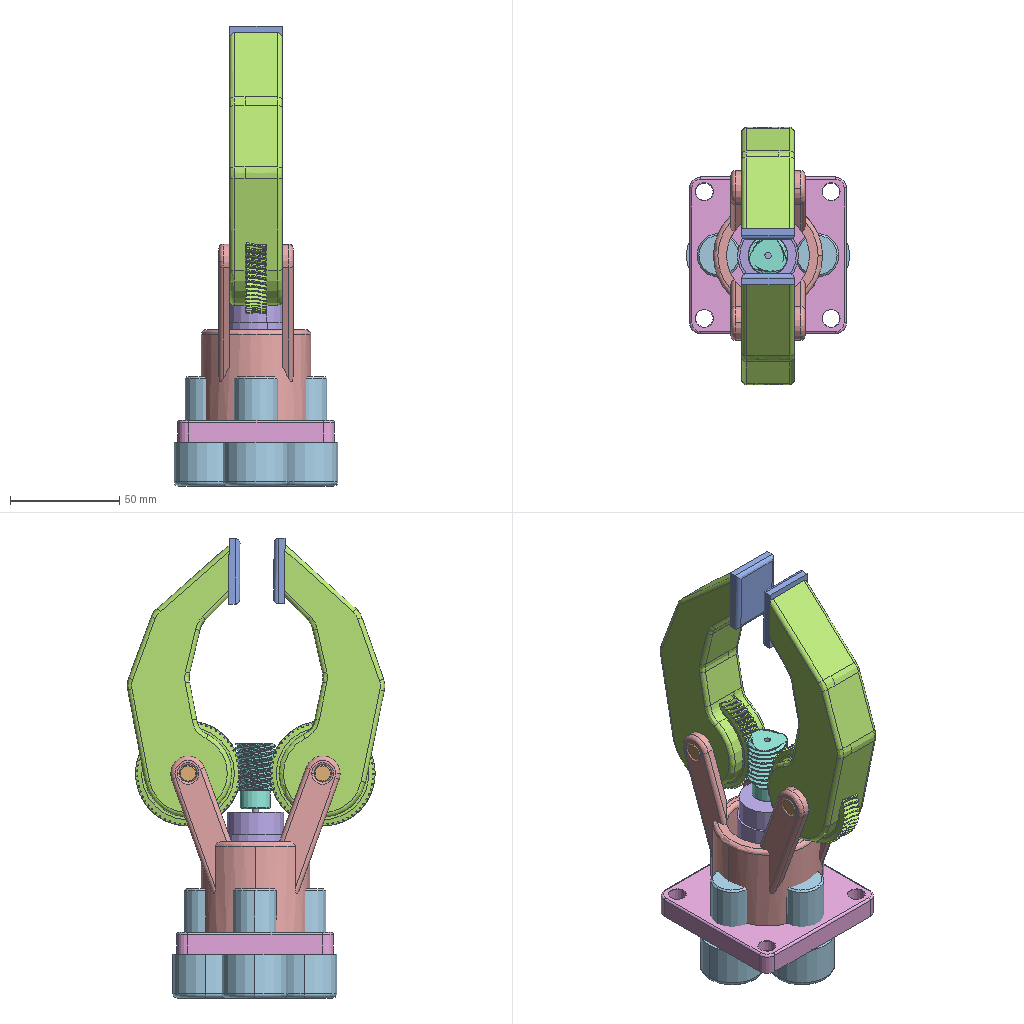Assembly | SolidWorks | 9 different items | 15 placed | box 75 x 118 x 211 mm
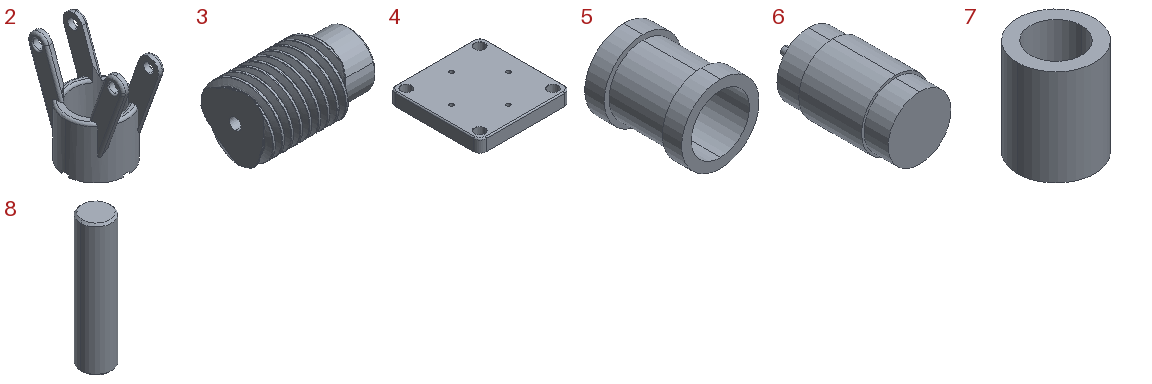Parts list (item | name | quantity | size | volume | features):
1 | - | x2 | - | - | features ICE 10, Fillet 3, CombineBodies 2, Chamfer 1, DeleteBody 1, MBimport 1, MirrorPattern 1
2 | - | x1 | 50 x 77.6 x 80.781 mm | 47492 mm3 | features ICE 7, Fillet 2, CirPattern 1, Extrusion 1, HoleWzd 1
3 | - | x1 | 30 x 18.04 x 18.04 mm | 5689 mm3 | features ICE 3, Chamfer 1, DeleteBody 1, MBimport 1
4 | - | x1 | 71.75 x 71.75 x 10 mm | 48903 mm3 | features Fillet 3, Extrusion 1, ICE 1
5 | - | x4 | 4 x 5 x 4 mm | 18.653 mm3 | features Revolution 1
6 | - | x1 | 28 x 56 x 28 mm | 26699 mm3 | features ICE 3, Extrusion 1
7 | - | x2 | 12 x 12 x 15 mm | 942.478 mm3 | features Extrusion 1
8 | - | x2 | 8 x 8 x 34 mm | 1703 mm3 | features Chamfer 1, Extrusion 1
9 | socket head cap screw 4762_din | x1 | - | - | -
Mates (type | each side: item.copy, entity, surface, feature):
Coincident | 2.1 face plane CirPattern1 | 1.1 face plane Boss-Extrude1
Coincident | 2.1 face plane Boss-Extrude4 | 1.2 face plane Boss-Extrude2
Concentric | 2.1 face cylinder CBORE for #5 Binding Head Machine Screw1 | 4.1 face cylinder Cut-Extrude1
Coincident | 2.1 face plane Cut-Extrude3 | 4.1 face plane Boss-Extrude1
Concentric | 2.1 face cylinder Boss-Extrude1 | 3.1 face cylinder Framo_Morat_3_60.stp
Coincident | 2.1 face plane CirPattern1 | 8.1 face plane Boss-Extrude1
Coincident | 2.1 face plane Boss-Extrude2 | 8.2 face plane Boss-Extrude1
Concentric | 2.1 face cylinder Boss-Extrude1 | 6.1 face cylinder Boss-Extrude2
Concentric | 2.1 face cylinder CBORE for #5 Binding Head Machine Screw1 | 5.1 face cylinder Revolve1
Coincident | 2.1 face plane CBORE for #5 Binding Head Machine Screw1 | 5.1 face plane Revolve1
Concentric | 2.1 face cylinder CBORE for #5 Binding Head Machine Screw1 | 5.2 face cylinder Revolve1
Coincident | 2.1 face plane CBORE for #5 Binding Head Machine Screw1 | 5.2 face plane Revolve1
Concentric | 2.1 face cylinder CBORE for #5 Binding Head Machine Screw1 | 5.3 face cylinder Revolve1
Coincident | 2.1 face plane CBORE for #5 Binding Head Machine Screw1 | 5.3 face plane Revolve1
Concentric | 2.1 face cylinder CBORE for #5 Binding Head Machine Screw1 | 5.4 face cylinder Revolve1
Coincident | 2.1 face plane CBORE for #5 Binding Head Machine Screw1 | 5.4 face plane Revolve1
Parallel | 4.1 plane | assembly plane
Concentric | 1.2 face cylinder Вырез-Вытянуть2 | 7.1 face cylinder Boss-Extrude1
Concentric | 1.1 face cylinder Вырез-Вытянуть2 | 7.2 face cylinder Boss-Extrude1
DistanceDim | 7.2 face plane Boss-Extrude1 | 1.1 face plane Boss-Extrude1
DistanceDim | 7.1 face plane Boss-Extrude1 | 1.2 face plane Boss-Extrude2
Concentric | 8.2 face cylinder Boss-Extrude1 | 7.1 face cylinder Boss-Extrude1
Concentric | 2.1 face cylinder Boss-Extrude4 | 8.2 face cylinder Boss-Extrude1
Concentric | 8.1 face cylinder Boss-Extrude1 | 7.2 face cylinder Boss-Extrude1
Concentric | 2.1 face cylinder CirPattern1 | 8.1 face cylinder Boss-Extrude1
Parallel | 1.1 face plane Boss-Extrude6 | 1.2 face plane Boss-Extrude6